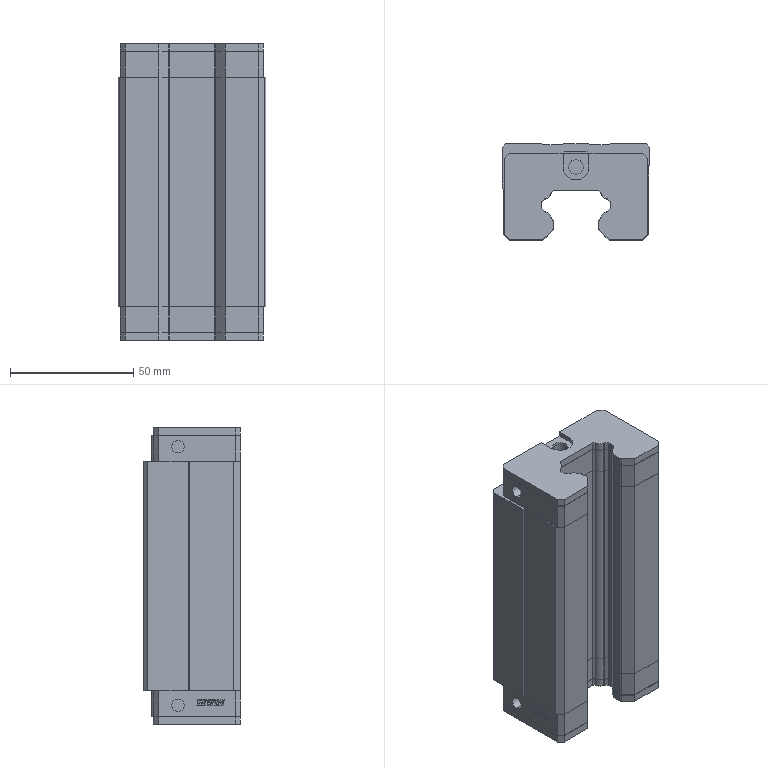Part | SolidWorks | features BaseBody 5 | 5 solids | 670 faces | box 60 x 39 x 120.4 mm | volume 211772 mm3 | plane 422 | cylinder 200 | cone 48 | commonest cylinder face diameters 1.2 x60 0.194 x34 1.6 x20 5.66 x20 0.097 x18 1 x8